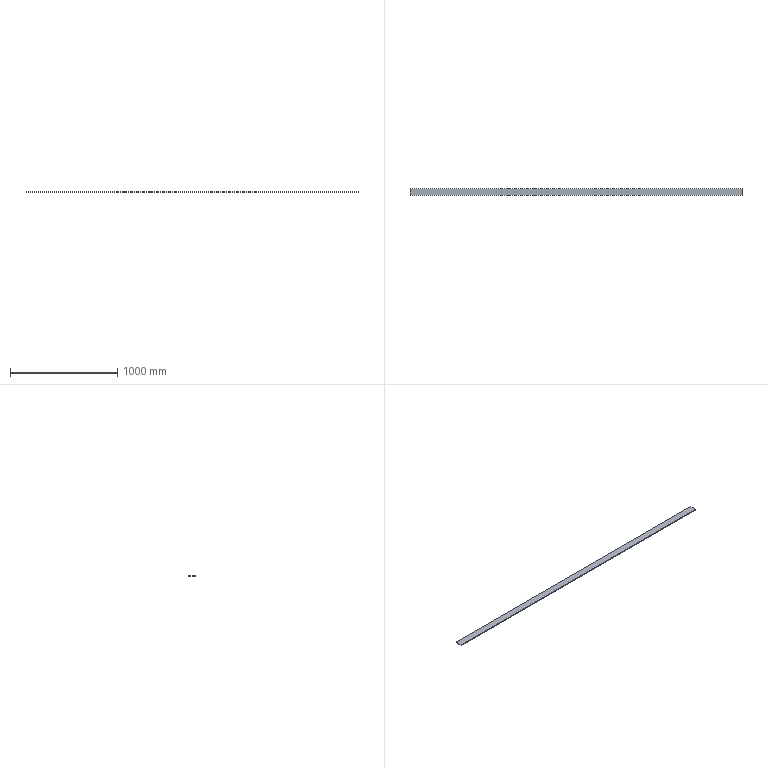Part | SolidWorks | features Extrusion 1 | 1 solid | 6 faces | box 3100 x 65 x 8 mm | volume 1612000 mm3 | plane 6
STEP:
#1=CARTESIAN_POINT('',(1550.,-32.5,0.));
#2=VERTEX_POINT('',#1);
#3=CARTESIAN_POINT('',(1550.,32.5,0.));
#4=VERTEX_POINT('',#3);
#5=CARTESIAN_POINT('',(1550.,-32.5,0.));
#6=DIRECTION('',(0.,1.,0.));
#7=VECTOR('',#6,1000.);
#8=LINE('',#5,#7);
#9=EDGE_CURVE('',#2,#4,#8,.T.);
#10=ORIENTED_EDGE('',*,*,#9,.T.);
#11=CARTESIAN_POINT('',(1550.,32.5,8.));
#12=VERTEX_POINT('',#11);
#13=CARTESIAN_POINT('',(1550.,32.5,8.));
#14=DIRECTION('',(0.,0.,-1.));
#15=VECTOR('',#14,1000.);
#16=LINE('',#13,#15);
#17=EDGE_CURVE('',#12,#4,#16,.T.);
#18=ORIENTED_EDGE('',*,*,#17,.F.);
#19=CARTESIAN_POINT('',(1550.,-32.5,8.));
#20=VERTEX_POINT('',#19);
#21=CARTESIAN_POINT('',(1550.,-32.5,8.));
#22=DIRECTION('',(0.,1.,0.));
#23=VECTOR('',#22,1000.);
#24=LINE('',#21,#23);
#25=EDGE_CURVE('',#20,#12,#24,.T.);
#26=ORIENTED_EDGE('',*,*,#25,.F.);
#27=CARTESIAN_POINT('',(1550.,-32.5,8.));
#28=DIRECTION('',(0.,0.,-1.));
#29=VECTOR('',#28,1000.);
#30=LINE('',#27,#29);
#31=EDGE_CURVE('',#20,#2,#30,.T.);
#32=ORIENTED_EDGE('',*,*,#31,.T.);
#33=EDGE_LOOP('',(#10,#18,#26,#32));
#34=FACE_OUTER_BOUND('',#33,.T.);
#35=CARTESIAN_POINT('',(1550.,-32.5,8.));
#36=DIRECTION('',(-1.,0.,0.));
#37=DIRECTION('',(0.,0.,1.));
#38=AXIS2_PLACEMENT_3D('',#35,#36,#37);
#39=PLANE('',#38);
#40=ADVANCED_FACE('',(#34),#39,.F.);
#41=CARTESIAN_POINT('',(-1550.,32.5,0.));
#42=VERTEX_POINT('',#41);
#43=CARTESIAN_POINT('',(-1550.,32.5,0.));
#44=DIRECTION('',(-1.,0.,0.));
#45=VECTOR('',#44,1000.);
#46=LINE('',#43,#45);
#47=EDGE_CURVE('',#4,#42,#46,.T.);
#48=ORIENTED_EDGE('',*,*,#47,.T.);
#49=CARTESIAN_POINT('',(-1550.,32.5,8.));
#50=VERTEX_POINT('',#49);
#51=CARTESIAN_POINT('',(-1550.,32.5,8.));
#52=DIRECTION('',(0.,0.,-1.));
#53=VECTOR('',#52,1000.);
#54=LINE('',#51,#53);
#55=EDGE_CURVE('',#50,#42,#54,.T.);
#56=ORIENTED_EDGE('',*,*,#55,.F.);
#57=CARTESIAN_POINT('',(-1550.,32.5,8.));
#58=DIRECTION('',(-1.,0.,0.));
#59=VECTOR('',#58,1000.);
#60=LINE('',#57,#59);
#61=EDGE_CURVE('',#12,#50,#60,.T.);
#62=ORIENTED_EDGE('',*,*,#61,.F.);
#63=ORIENTED_EDGE('',*,*,#17,.T.);
#64=EDGE_LOOP('',(#48,#56,#62,#63));
#65=FACE_OUTER_BOUND('',#64,.T.);
#66=CARTESIAN_POINT('',(-1550.,32.5,8.));
#67=DIRECTION('',(0.,-1.,0.));
#68=DIRECTION('',(0.,0.,-1.));
#69=AXIS2_PLACEMENT_3D('',#66,#67,#68);
#70=PLANE('',#69);
#71=ADVANCED_FACE('',(#65),#70,.F.);
#72=CARTESIAN_POINT('',(-1550.,-32.5,0.));
#73=VERTEX_POINT('',#72);
#74=CARTESIAN_POINT('',(-1550.,-32.5,0.));
#75=DIRECTION('',(0.,-1.,0.));
#76=VECTOR('',#75,1000.);
#77=LINE('',#74,#76);
#78=EDGE_CURVE('',#42,#73,#77,.T.);
#79=ORIENTED_EDGE('',*,*,#78,.T.);
#80=CARTESIAN_POINT('',(-1550.,-32.5,8.));
#81=VERTEX_POINT('',#80);
#82=CARTESIAN_POINT('',(-1550.,-32.5,8.));
#83=DIRECTION('',(0.,0.,-1.));
#84=VECTOR('',#83,1000.);
#85=LINE('',#82,#84);
#86=EDGE_CURVE('',#81,#73,#85,.T.);
#87=ORIENTED_EDGE('',*,*,#86,.F.);
#88=CARTESIAN_POINT('',(-1550.,-32.5,8.));
#89=DIRECTION('',(0.,-1.,0.));
#90=VECTOR('',#89,1000.);
#91=LINE('',#88,#90);
#92=EDGE_CURVE('',#50,#81,#91,.T.);
#93=ORIENTED_EDGE('',*,*,#92,.F.);
#94=ORIENTED_EDGE('',*,*,#55,.T.);
#95=EDGE_LOOP('',(#79,#87,#93,#94));
#96=FACE_OUTER_BOUND('',#95,.T.);
#97=CARTESIAN_POINT('',(-1550.,-32.5,8.));
#98=DIRECTION('',(1.,0.,0.));
#99=DIRECTION('',(0.,0.,-1.));
#100=AXIS2_PLACEMENT_3D('',#97,#98,#99);
#101=PLANE('',#100);
#102=ADVANCED_FACE('',(#96),#101,.F.);
#103=CARTESIAN_POINT('',(-1550.,-32.5,0.));
#104=DIRECTION('',(1.,0.,0.));
#105=VECTOR('',#104,1000.);
#106=LINE('',#103,#105);
#107=EDGE_CURVE('',#73,#2,#106,.T.);
#108=ORIENTED_EDGE('',*,*,#107,.T.);
#109=ORIENTED_EDGE('',*,*,#31,.F.);
#110=CARTESIAN_POINT('',(-1550.,-32.5,8.));
#111=DIRECTION('',(1.,0.,0.));
#112=VECTOR('',#111,1000.);
#113=LINE('',#110,#112);
#114=EDGE_CURVE('',#81,#20,#113,.T.);
#115=ORIENTED_EDGE('',*,*,#114,.F.);
#116=ORIENTED_EDGE('',*,*,#86,.T.);
#117=EDGE_LOOP('',(#108,#109,#115,#116));
#118=FACE_OUTER_BOUND('',#117,.T.);
#119=CARTESIAN_POINT('',(-1550.,-32.5,8.));
#120=DIRECTION('',(0.,1.,0.));
#121=DIRECTION('',(0.,0.,1.));
#122=AXIS2_PLACEMENT_3D('',#119,#120,#121);
#123=PLANE('',#122);
#124=ADVANCED_FACE('',(#118),#123,.F.);
#125=ORIENTED_EDGE('',*,*,#25,.T.);
#126=ORIENTED_EDGE('',*,*,#61,.T.);
#127=ORIENTED_EDGE('',*,*,#92,.T.);
#128=ORIENTED_EDGE('',*,*,#114,.T.);
#129=EDGE_LOOP('',(#125,#126,#127,#128));
#130=FACE_OUTER_BOUND('',#129,.T.);
#131=CARTESIAN_POINT('',(0.,0.,8.));
#132=DIRECTION('',(0.,0.,-1.));
#133=DIRECTION('',(-1.,0.,0.));
#134=AXIS2_PLACEMENT_3D('',#131,#132,#133);
#135=PLANE('',#134);
#136=ADVANCED_FACE('',(#130),#135,.F.);
#137=ORIENTED_EDGE('',*,*,#9,.F.);
#138=ORIENTED_EDGE('',*,*,#107,.F.);
#139=ORIENTED_EDGE('',*,*,#78,.F.);
#140=ORIENTED_EDGE('',*,*,#47,.F.);
#141=EDGE_LOOP('',(#137,#138,#139,#140));
#142=FACE_OUTER_BOUND('',#141,.T.);
#143=CARTESIAN_POINT('',(0.,0.,0.));
#144=DIRECTION('',(0.,0.,-1.));
#145=DIRECTION('',(-1.,0.,0.));
#146=AXIS2_PLACEMENT_3D('',#143,#144,#145);
#147=PLANE('',#146);
#148=ADVANCED_FACE('',(#142),#147,.T.);
#149=CLOSED_SHELL('',(#40,#71,#102,#124,#136,#148));
#150=MANIFOLD_SOLID_BREP('',#149);
#151=CARTESIAN_POINT('',(0.,0.,0.));
#152=DIRECTION('',(0.,0.,1.));
#153=DIRECTION('',(1.,0.,0.));
#154=AXIS2_PLACEMENT_3D('',#151,#152,#153);
#155=(LENGTH_UNIT()NAMED_UNIT(*)SI_UNIT(.MILLI.,.METRE.));
#156=UNCERTAINTY_MEASURE_WITH_UNIT(LENGTH_MEASURE(0.00001),#155,'','');
#157=(NAMED_UNIT(*)PLANE_ANGLE_UNIT()SI_UNIT($,.RADIAN.));
#158=(NAMED_UNIT(*)SI_UNIT($,.STERADIAN.)SOLID_ANGLE_UNIT());
#159=(GEOMETRIC_REPRESENTATION_CONTEXT(3)GLOBAL_UNCERTAINTY_ASSIGNED_CONTEXT((#156))GLOBAL_UNIT_ASSIGNED_CONTEXT((#155,#157,#158))REPRESENTATION_CONTEXT('',''));
#160=ADVANCED_BREP_SHAPE_REPRESENTATION('',(#150,#154),#159);